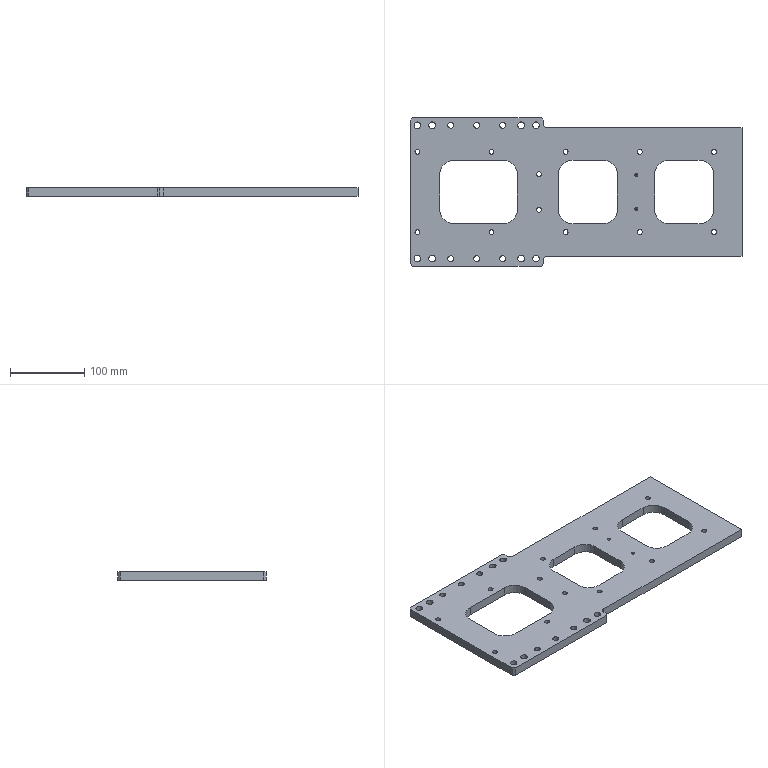Part | STEP file | J454-EBZ05-01-04-Part-1 | 1 solid | 180 faces | box 448 x 200 x 12 mm | volume 706268 mm3 | cylinder 122 | plane 46 | cone 12 | commonest cylinder face diameters 6.6 x24 11 x24 8 x16 9 x16 40 x12 5.1 x8